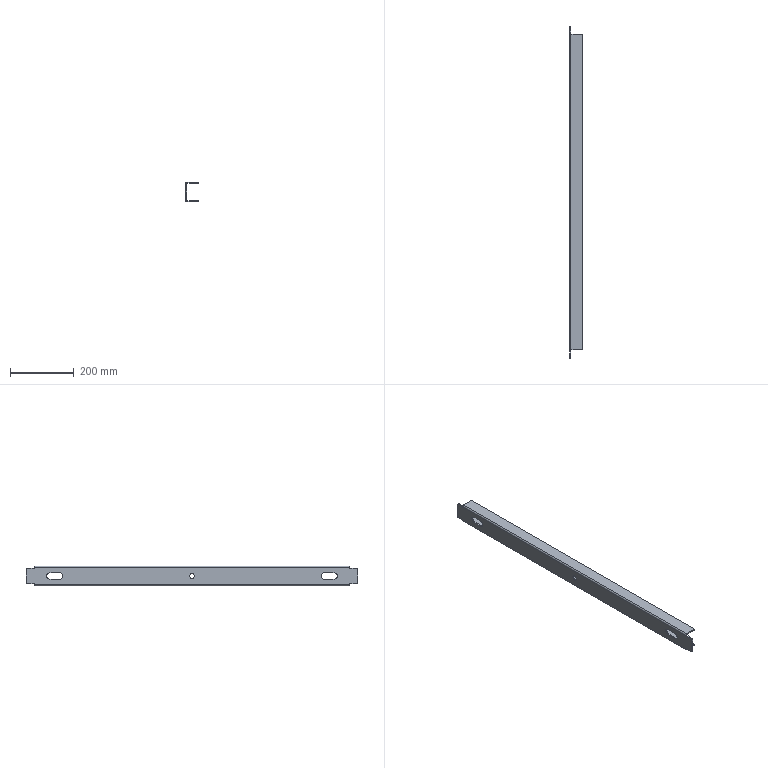Part | SolidWorks | features SMBaseFlange 2, Cut 1, Fillet 1, FlatPattern 1, SheetMetal 1 | 1 solid | 44 faces | box 40 x 1040 x 62 mm | volume 524399 mm3 | plane 30 | cylinder 14 | commonest cylinder face diameters 10 x4 20 x4 0.4 x2 8.4 x2 15 x2
STEP:
#1=CARTESIAN_POINT('',(0.,0.,-7.5));
#2=VERTEX_POINT('',#1);
#3=CARTESIAN_POINT('',(0.,0.,7.5));
#4=VERTEX_POINT('',#3);
#5=CARTESIAN_POINT('',(0.,0.,0.));
#6=DIRECTION('',(-1.,0.,0.));
#7=DIRECTION('',(0.,0.,1.));
#8=AXIS2_PLACEMENT_3D('',#5,#6,#7);
#9=CIRCLE('',#8,7.5);
#10=EDGE_CURVE('',#2,#4,#9,.T.);
#11=ORIENTED_EDGE('',*,*,#10,.T.);
#12=CARTESIAN_POINT('',(4.,0.,7.5));
#13=VERTEX_POINT('',#12);
#14=CARTESIAN_POINT('',(-6.,0.,7.5));
#15=DIRECTION('',(1.,0.,0.));
#16=VECTOR('',#15,1000.);
#17=LINE('',#14,#16);
#18=EDGE_CURVE('',#4,#13,#17,.T.);
#19=ORIENTED_EDGE('',*,*,#18,.T.);
#20=CARTESIAN_POINT('',(4.,0.,-7.5));
#21=VERTEX_POINT('',#20);
#22=CARTESIAN_POINT('',(4.,0.,0.));
#23=DIRECTION('',(1.,0.,0.));
#24=DIRECTION('',(0.,0.,-1.));
#25=AXIS2_PLACEMENT_3D('',#22,#23,#24);
#26=CIRCLE('',#25,7.5);
#27=EDGE_CURVE('',#13,#21,#26,.T.);
#28=ORIENTED_EDGE('',*,*,#27,.T.);
#29=CARTESIAN_POINT('',(-6.,0.,-7.5));
#30=DIRECTION('',(1.,0.,0.));
#31=VECTOR('',#30,1000.);
#32=LINE('',#29,#31);
#33=EDGE_CURVE('',#2,#21,#32,.T.);
#34=ORIENTED_EDGE('',*,*,#33,.F.);
#35=EDGE_LOOP('',(#11,#19,#28,#34));
#36=FACE_OUTER_BOUND('',#35,.T.);
#37=CARTESIAN_POINT('',(-6.,0.,0.));
#38=DIRECTION('',(1.,0.,0.));
#39=DIRECTION('',(0.,0.,-1.));
#40=AXIS2_PLACEMENT_3D('',#37,#38,#39);
#41=CYLINDRICAL_SURFACE('',#40,7.5);
#42=ADVANCED_FACE('',(#36),#41,.F.);
#43=CARTESIAN_POINT('',(4.,-494.,25.));
#44=VERTEX_POINT('',#43);
#45=CARTESIAN_POINT('',(0.,-494.,25.));
#46=VERTEX_POINT('',#45);
#47=CARTESIAN_POINT('',(4.2,-494.,25.));
#48=DIRECTION('',(-1.,0.,0.));
#49=VECTOR('',#48,1000.);
#50=LINE('',#47,#49);
#51=EDGE_CURVE('',#44,#46,#50,.T.);
#52=ORIENTED_EDGE('',*,*,#51,.F.);
#53=CARTESIAN_POINT('',(4.,-494.,26.8));
#54=VERTEX_POINT('',#53);
#55=CARTESIAN_POINT('',(4.,-494.,-31.));
#56=DIRECTION('',(0.,0.,-1.));
#57=VECTOR('',#56,1000.);
#58=LINE('',#55,#57);
#59=EDGE_CURVE('',#54,#44,#58,.T.);
#60=ORIENTED_EDGE('',*,*,#59,.F.);
#61=CARTESIAN_POINT('',(0.,-494.,26.8));
#62=VERTEX_POINT('',#61);
#63=CARTESIAN_POINT('',(4.,-494.,26.8));
#64=DIRECTION('',(-1.,0.,0.));
#65=VECTOR('',#64,1000.);
#66=LINE('',#63,#65);
#67=EDGE_CURVE('',#54,#62,#66,.T.);
#68=ORIENTED_EDGE('',*,*,#67,.T.);
#69=CARTESIAN_POINT('',(0.,-494.,-31.));
#70=DIRECTION('',(0.,0.,-1.));
#71=VECTOR('',#70,1000.);
#72=LINE('',#69,#71);
#73=EDGE_CURVE('',#62,#46,#72,.T.);
#74=ORIENTED_EDGE('',*,*,#73,.T.);
#75=EDGE_LOOP('',(#52,#60,#68,#74));
#76=FACE_OUTER_BOUND('',#75,.T.);
#77=CARTESIAN_POINT('',(4.2,-494.,-27.));
#78=DIRECTION('',(0.,-1.,0.));
#79=DIRECTION('',(0.,0.,-1.));
#80=AXIS2_PLACEMENT_3D('',#77,#78,#79);
#81=PLANE('',#80);
#82=ADVANCED_FACE('',(#76),#81,.T.);
#83=CARTESIAN_POINT('',(4.,494.,-25.));
#84=VERTEX_POINT('',#83);
#85=CARTESIAN_POINT('',(0.,494.,-25.));
#86=VERTEX_POINT('',#85);
#87=CARTESIAN_POINT('',(4.2,494.,-25.));
#88=DIRECTION('',(-1.,0.,0.));
#89=VECTOR('',#88,1000.);
#90=LINE('',#87,#89);
#91=EDGE_CURVE('',#84,#86,#90,.T.);
#92=ORIENTED_EDGE('',*,*,#91,.F.);
#93=CARTESIAN_POINT('',(4.,494.,-26.8));
#94=VERTEX_POINT('',#93);
#95=CARTESIAN_POINT('',(4.,494.,-31.));
#96=DIRECTION('',(0.,0.,-1.));
#97=VECTOR('',#96,1000.);
#98=LINE('',#95,#97);
#99=EDGE_CURVE('',#84,#94,#98,.T.);
#100=ORIENTED_EDGE('',*,*,#99,.T.);
#101=CARTESIAN_POINT('',(0.,494.,-26.8));
#102=VERTEX_POINT('',#101);
#103=CARTESIAN_POINT('',(4.,494.,-26.8));
#104=DIRECTION('',(-1.,0.,0.));
#105=VECTOR('',#104,1000.);
#106=LINE('',#103,#105);
#107=EDGE_CURVE('',#94,#102,#106,.T.);
#108=ORIENTED_EDGE('',*,*,#107,.T.);
#109=CARTESIAN_POINT('',(0.,494.,-31.));
#110=DIRECTION('',(0.,0.,-1.));
#111=VECTOR('',#110,1000.);
#112=LINE('',#109,#111);
#113=EDGE_CURVE('',#86,#102,#112,.T.);
#114=ORIENTED_EDGE('',*,*,#113,.F.);
#115=EDGE_LOOP('',(#92,#100,#108,#114));
#116=FACE_OUTER_BOUND('',#115,.T.);
#117=CARTESIAN_POINT('',(4.2,494.,27.));
#118=DIRECTION('',(0.,1.,0.));
#119=DIRECTION('',(0.,0.,1.));
#120=AXIS2_PLACEMENT_3D('',#117,#118,#119);
#121=PLANE('',#120);
#122=ADVANCED_FACE('',(#116),#121,.T.);
#123=CARTESIAN_POINT('',(0.,494.,26.8));
#124=VERTEX_POINT('',#123);
#125=CARTESIAN_POINT('',(4.,494.,26.8));
#126=VERTEX_POINT('',#125);
#127=CARTESIAN_POINT('',(0.,494.,26.8));
#128=DIRECTION('',(1.,0.,0.));
#129=VECTOR('',#128,1000.);
#130=LINE('',#127,#129);
#131=EDGE_CURVE('',#124,#126,#130,.T.);
#132=ORIENTED_EDGE('',*,*,#131,.F.);
#133=CARTESIAN_POINT('',(4.2,494.,31.));
#134=VERTEX_POINT('',#133);
#135=CARTESIAN_POINT('',(4.2,494.,26.8));
#136=DIRECTION('',(0.,-1.,0.));
#137=DIRECTION('',(0.,0.,1.));
#138=AXIS2_PLACEMENT_3D('',#135,#136,#137);
#139=CIRCLE('',#138,4.2);
#140=EDGE_CURVE('',#134,#124,#139,.T.);
#141=ORIENTED_EDGE('',*,*,#140,.F.);
#142=CARTESIAN_POINT('',(4.2,494.,27.));
#143=VERTEX_POINT('',#142);
#144=CARTESIAN_POINT('',(4.2,494.,27.));
#145=DIRECTION('',(0.,0.,1.));
#146=VECTOR('',#145,1000.);
#147=LINE('',#144,#146);
#148=EDGE_CURVE('',#143,#134,#147,.T.);
#149=ORIENTED_EDGE('',*,*,#148,.F.);
#150=CARTESIAN_POINT('',(4.2,494.,26.8));
#151=DIRECTION('',(0.,-1.,0.));
#152=DIRECTION('',(1.,0.,0.));
#153=AXIS2_PLACEMENT_3D('',#150,#151,#152);
#154=CIRCLE('',#153,0.2);
#155=EDGE_CURVE('',#143,#126,#154,.T.);
#156=ORIENTED_EDGE('',*,*,#155,.T.);
#157=EDGE_LOOP('',(#132,#141,#149,#156));
#158=FACE_OUTER_BOUND('',#157,.T.);
#159=CARTESIAN_POINT('',(0.,494.,26.8));
#160=DIRECTION('',(0.,1.,0.));
#161=DIRECTION('',(0.,0.,1.));
#162=AXIS2_PLACEMENT_3D('',#159,#160,#161);
#163=PLANE('',#162);
#164=ADVANCED_FACE('',(#158),#163,.T.);
#165=CARTESIAN_POINT('',(0.,494.,25.));
#166=VERTEX_POINT('',#165);
#167=CARTESIAN_POINT('',(4.,494.,25.));
#168=VERTEX_POINT('',#167);
#169=CARTESIAN_POINT('',(4.2,494.,25.));
#170=DIRECTION('',(1.,0.,0.));
#171=VECTOR('',#170,1000.);
#172=LINE('',#169,#171);
#173=EDGE_CURVE('',#166,#168,#172,.T.);
#174=ORIENTED_EDGE('',*,*,#173,.F.);
#175=CARTESIAN_POINT('',(0.,494.,-31.));
#176=DIRECTION('',(0.,0.,-1.));
#177=VECTOR('',#176,1000.);
#178=LINE('',#175,#177);
#179=EDGE_CURVE('',#124,#166,#178,.T.);
#180=ORIENTED_EDGE('',*,*,#179,.F.);
#181=ORIENTED_EDGE('',*,*,#131,.T.);
#182=CARTESIAN_POINT('',(4.,494.,-31.));
#183=DIRECTION('',(0.,0.,-1.));
#184=VECTOR('',#183,1000.);
#185=LINE('',#182,#184);
#186=EDGE_CURVE('',#126,#168,#185,.T.);
#187=ORIENTED_EDGE('',*,*,#186,.T.);
#188=EDGE_LOOP('',(#174,#180,#181,#187));
#189=FACE_OUTER_BOUND('',#188,.T.);
#190=CARTESIAN_POINT('',(4.2,494.,27.));
#191=DIRECTION('',(0.,1.,0.));
#192=DIRECTION('',(0.,0.,1.));
#193=AXIS2_PLACEMENT_3D('',#190,#191,#192);
#194=PLANE('',#193);
#195=ADVANCED_FACE('',(#189),#194,.T.);
#196=CARTESIAN_POINT('',(4.2,-494.,31.));
#197=VERTEX_POINT('',#196);
#198=CARTESIAN_POINT('',(4.2,-494.,27.));
#199=VERTEX_POINT('',#198);
#200=CARTESIAN_POINT('',(4.2,-494.,31.));
#201=DIRECTION('',(0.,0.,-1.));
#202=VECTOR('',#201,1000.);
#203=LINE('',#200,#202);
#204=EDGE_CURVE('',#197,#199,#203,.T.);
#205=ORIENTED_EDGE('',*,*,#204,.F.);
#206=CARTESIAN_POINT('',(4.2,-494.,26.8));
#207=DIRECTION('',(0.,-1.,0.));
#208=DIRECTION('',(0.,0.,1.));
#209=AXIS2_PLACEMENT_3D('',#206,#207,#208);
#210=CIRCLE('',#209,4.2);
#211=EDGE_CURVE('',#197,#62,#210,.T.);
#212=ORIENTED_EDGE('',*,*,#211,.T.);
#213=ORIENTED_EDGE('',*,*,#67,.F.);
#214=CARTESIAN_POINT('',(4.2,-494.,26.8));
#215=DIRECTION('',(0.,-1.,0.));
#216=DIRECTION('',(1.,0.,0.));
#217=AXIS2_PLACEMENT_3D('',#214,#215,#216);
#218=CIRCLE('',#217,0.2);
#219=EDGE_CURVE('',#199,#54,#218,.T.);
#220=ORIENTED_EDGE('',*,*,#219,.F.);
#221=EDGE_LOOP('',(#205,#212,#213,#220));
#222=FACE_OUTER_BOUND('',#221,.T.);
#223=CARTESIAN_POINT('',(4.2,-494.,31.));
#224=DIRECTION('',(0.,-1.,0.));
#225=DIRECTION('',(0.,0.,-1.));
#226=AXIS2_PLACEMENT_3D('',#223,#224,#225);
#227=PLANE('',#226);
#228=ADVANCED_FACE('',(#222),#227,.T.);
#229=CARTESIAN_POINT('',(40.,-494.,31.));
#230=VERTEX_POINT('',#229);
#231=CARTESIAN_POINT('',(0.,-494.,31.));
#232=DIRECTION('',(-1.,0.,0.));
#233=VECTOR('',#232,1000.);
#234=LINE('',#231,#233);
#235=EDGE_CURVE('',#230,#197,#234,.T.);
#236=ORIENTED_EDGE('',*,*,#235,.T.);
#237=ORIENTED_EDGE('',*,*,#204,.T.);
#238=CARTESIAN_POINT('',(40.,-494.,27.));
#239=VERTEX_POINT('',#238);
#240=CARTESIAN_POINT('',(0.,-494.,27.));
#241=DIRECTION('',(-1.,0.,0.));
#242=VECTOR('',#241,1000.);
#243=LINE('',#240,#242);
#244=EDGE_CURVE('',#239,#199,#243,.T.);
#245=ORIENTED_EDGE('',*,*,#244,.F.);
#246=CARTESIAN_POINT('',(40.,-494.,27.));
#247=DIRECTION('',(0.,0.,1.));
#248=VECTOR('',#247,1000.);
#249=LINE('',#246,#248);
#250=EDGE_CURVE('',#239,#230,#249,.T.);
#251=ORIENTED_EDGE('',*,*,#250,.T.);
#252=EDGE_LOOP('',(#236,#237,#245,#251));
#253=FACE_OUTER_BOUND('',#252,.T.);
#254=CARTESIAN_POINT('',(4.,-494.,26.8));
#255=DIRECTION('',(0.,-1.,0.));
#256=DIRECTION('',(0.,0.,-1.));
#257=AXIS2_PLACEMENT_3D('',#254,#255,#256);
#258=PLANE('',#257);
#259=ADVANCED_FACE('',(#253),#258,.T.);
#260=CARTESIAN_POINT('',(4.2,494.,-31.));
#261=VERTEX_POINT('',#260);
#262=CARTESIAN_POINT('',(4.2,494.,-27.));
#263=VERTEX_POINT('',#262);
#264=CARTESIAN_POINT('',(4.2,494.,-31.));
#265=DIRECTION('',(0.,0.,1.));
#266=VECTOR('',#265,1000.);
#267=LINE('',#264,#266);
#268=EDGE_CURVE('',#261,#263,#267,.T.);
#269=ORIENTED_EDGE('',*,*,#268,.F.);
#270=CARTESIAN_POINT('',(4.2,494.,-26.8));
#271=DIRECTION('',(0.,-1.,0.));
#272=DIRECTION('',(0.,0.,1.));
#273=AXIS2_PLACEMENT_3D('',#270,#271,#272);
#274=CIRCLE('',#273,4.2);
#275=EDGE_CURVE('',#102,#261,#274,.T.);
#276=ORIENTED_EDGE('',*,*,#275,.F.);
#277=ORIENTED_EDGE('',*,*,#107,.F.);
#278=CARTESIAN_POINT('',(4.2,494.,-26.8));
#279=DIRECTION('',(0.,-1.,0.));
#280=DIRECTION('',(1.,0.,0.));
#281=AXIS2_PLACEMENT_3D('',#278,#279,#280);
#282=CIRCLE('',#281,0.2);
#283=EDGE_CURVE('',#94,#263,#282,.T.);
#284=ORIENTED_EDGE('',*,*,#283,.T.);
#285=EDGE_LOOP('',(#269,#276,#277,#284));
#286=FACE_OUTER_BOUND('',#285,.T.);
#287=CARTESIAN_POINT('',(4.2,494.,-31.));
#288=DIRECTION('',(0.,1.,0.));
#289=DIRECTION('',(0.,0.,1.));
#290=AXIS2_PLACEMENT_3D('',#287,#288,#289);
#291=PLANE('',#290);
#292=ADVANCED_FACE('',(#286),#291,.T.);
#293=CARTESIAN_POINT('',(40.,494.,-31.));
#294=VERTEX_POINT('',#293);
#295=CARTESIAN_POINT('',(0.,494.,-31.));
#296=DIRECTION('',(1.,0.,0.));
#297=VECTOR('',#296,1000.);
#298=LINE('',#295,#297);
#299=EDGE_CURVE('',#261,#294,#298,.T.);
#300=ORIENTED_EDGE('',*,*,#299,.F.);
#301=ORIENTED_EDGE('',*,*,#268,.T.);
#302=CARTESIAN_POINT('',(40.,494.,-27.));
#303=VERTEX_POINT('',#302);
#304=CARTESIAN_POINT('',(0.,494.,-27.));
#305=DIRECTION('',(1.,0.,0.));
#306=VECTOR('',#305,1000.);
#307=LINE('',#304,#306);
#308=EDGE_CURVE('',#263,#303,#307,.T.);
#309=ORIENTED_EDGE('',*,*,#308,.T.);
#310=CARTESIAN_POINT('',(40.,494.,-31.));
#311=DIRECTION('',(0.,0.,1.));
#312=VECTOR('',#311,1000.);
#313=LINE('',#310,#312);
#314=EDGE_CURVE('',#294,#303,#313,.T.);
#315=ORIENTED_EDGE('',*,*,#314,.F.);
#316=EDGE_LOOP('',(#300,#301,#309,#315));
#317=FACE_OUTER_BOUND('',#316,.T.);
#318=CARTESIAN_POINT('',(4.,494.,-26.8));
#319=DIRECTION('',(0.,1.,0.));
#320=DIRECTION('',(0.,0.,1.));
#321=AXIS2_PLACEMENT_3D('',#318,#319,#320);
#322=PLANE('',#321);
#323=ADVANCED_FACE('',(#317),#322,.T.);
#324=CARTESIAN_POINT('',(0.,-494.,-26.8));
#325=VERTEX_POINT('',#324);
#326=CARTESIAN_POINT('',(4.,-494.,-26.8));
#327=VERTEX_POINT('',#326);
#328=CARTESIAN_POINT('',(0.,-494.,-26.8));
#329=DIRECTION('',(1.,0.,0.));
#330=VECTOR('',#329,1000.);
#331=LINE('',#328,#330);
#332=EDGE_CURVE('',#325,#327,#331,.T.);
#333=ORIENTED_EDGE('',*,*,#332,.F.);
#334=CARTESIAN_POINT('',(4.2,-494.,-31.));
#335=VERTEX_POINT('',#334);
#336=CARTESIAN_POINT('',(4.2,-494.,-26.8));
#337=DIRECTION('',(0.,-1.,0.));
#338=DIRECTION('',(0.,0.,1.));
#339=AXIS2_PLACEMENT_3D('',#336,#337,#338);
#340=CIRCLE('',#339,4.2);
#341=EDGE_CURVE('',#325,#335,#340,.T.);
#342=ORIENTED_EDGE('',*,*,#341,.T.);
#343=CARTESIAN_POINT('',(4.2,-494.,-27.));
#344=VERTEX_POINT('',#343);
#345=CARTESIAN_POINT('',(4.2,-494.,-27.));
#346=DIRECTION('',(0.,0.,-1.));
#347=VECTOR('',#346,1000.);
#348=LINE('',#345,#347);
#349=EDGE_CURVE('',#344,#335,#348,.T.);
#350=ORIENTED_EDGE('',*,*,#349,.F.);
#351=CARTESIAN_POINT('',(4.2,-494.,-26.8));
#352=DIRECTION('',(0.,-1.,0.));
#353=DIRECTION('',(1.,0.,0.));
#354=AXIS2_PLACEMENT_3D('',#351,#352,#353);
#355=CIRCLE('',#354,0.2);
#356=EDGE_CURVE('',#327,#344,#355,.T.);
#357=ORIENTED_EDGE('',*,*,#356,.F.);
#358=EDGE_LOOP('',(#333,#342,#350,#357));
#359=FACE_OUTER_BOUND('',#358,.T.);
#360=CARTESIAN_POINT('',(0.,-494.,-26.8));
#361=DIRECTION('',(0.,-1.,0.));
#362=DIRECTION('',(0.,0.,-1.));
#363=AXIS2_PLACEMENT_3D('',#360,#361,#362);
#364=PLANE('',#363);
#365=ADVANCED_FACE('',(#359),#364,.T.);
#366=CARTESIAN_POINT('',(0.,-494.,-25.));
#367=VERTEX_POINT('',#366);
#368=CARTESIAN_POINT('',(4.,-494.,-25.));
#369=VERTEX_POINT('',#368);
#370=CARTESIAN_POINT('',(4.2,-494.,-25.));
#371=DIRECTION('',(1.,0.,0.));
#372=VECTOR('',#371,1000.);
#373=LINE('',#370,#372);
#374=EDGE_CURVE('',#367,#369,#373,.T.);
#375=ORIENTED_EDGE('',*,*,#374,.F.);
#376=CARTESIAN_POINT('',(0.,-494.,-31.));
#377=DIRECTION('',(0.,0.,-1.));
#378=VECTOR('',#377,1000.);
#379=LINE('',#376,#378);
#380=EDGE_CURVE('',#367,#325,#379,.T.);
#381=ORIENTED_EDGE('',*,*,#380,.T.);
#382=ORIENTED_EDGE('',*,*,#332,.T.);
#383=CARTESIAN_POINT('',(4.,-494.,-31.));
#384=DIRECTION('',(0.,0.,-1.));
#385=VECTOR('',#384,1000.);
#386=LINE('',#383,#385);
#387=EDGE_CURVE('',#369,#327,#386,.T.);
#388=ORIENTED_EDGE('',*,*,#387,.F.);
#389=EDGE_LOOP('',(#375,#381,#382,#388));
#390=FACE_OUTER_BOUND('',#389,.T.);
#391=CARTESIAN_POINT('',(4.2,-494.,-27.));
#392=DIRECTION('',(0.,-1.,0.));
#393=DIRECTION('',(0.,0.,-1.));
#394=AXIS2_PLACEMENT_3D('',#391,#392,#393);
#395=PLANE('',#394);
#396=ADVANCED_FACE('',(#390),#395,.T.);
#397=CARTESIAN_POINT('',(40.,-494.,-27.));
#398=VERTEX_POINT('',#397);
#399=CARTESIAN_POINT('',(0.,-494.,-27.));
#400=DIRECTION('',(1.,0.,0.));
#401=VECTOR('',#400,1000.);
#402=LINE('',#399,#401);
#403=EDGE_CURVE('',#344,#398,#402,.T.);
#404=ORIENTED_EDGE('',*,*,#403,.T.);
#405=CARTESIAN_POINT('',(40.,494.,-27.));
#406=DIRECTION('',(0.,-1.,0.));
#407=VECTOR('',#406,1000.);
#408=LINE('',#405,#407);
#409=EDGE_CURVE('',#303,#398,#408,.T.);
#410=ORIENTED_EDGE('',*,*,#409,.F.);
#411=ORIENTED_EDGE('',*,*,#308,.F.);
#412=CARTESIAN_POINT('',(4.2,494.,-27.));
#413=DIRECTION('',(0.,-1.,0.));
#414=VECTOR('',#413,1000.);
#415=LINE('',#412,#414);
#416=EDGE_CURVE('',#263,#344,#415,.T.);
#417=ORIENTED_EDGE('',*,*,#416,.T.);
#418=EDGE_LOOP('',(#404,#410,#411,#417));
#419=FACE_OUTER_BOUND('',#418,.T.);
#420=CARTESIAN_POINT('',(0.,494.,-27.));
#421=DIRECTION('',(0.,0.,-1.));
#422=DIRECTION('',(-1.,0.,0.));
#423=AXIS2_PLACEMENT_3D('',#420,#421,#422);
#424=PLANE('',#423);
#425=ADVANCED_FACE('',(#419),#424,.F.);
#426=CARTESIAN_POINT('',(40.,-494.,-31.));
#427=VERTEX_POINT('',#426);
#428=CARTESIAN_POINT('',(40.,-494.,-31.));
#429=DIRECTION('',(0.,0.,1.));
#430=VECTOR('',#429,1000.);
#431=LINE('',#428,#430);
#432=EDGE_CURVE('',#427,#398,#431,.T.);
#433=ORIENTED_EDGE('',*,*,#432,.F.);
#434=CARTESIAN_POINT('',(40.,494.,-31.));
#435=DIRECTION('',(0.,-1.,0.));
#436=VECTOR('',#435,1000.);
#437=LINE('',#434,#436);
#438=EDGE_CURVE('',#294,#427,#437,.T.);
#439=ORIENTED_EDGE('',*,*,#438,.F.);
#440=ORIENTED_EDGE('',*,*,#314,.T.);
#441=ORIENTED_EDGE('',*,*,#409,.T.);
#442=EDGE_LOOP('',(#433,#439,#440,#441));
#443=FACE_OUTER_BOUND('',#442,.T.);
#444=CARTESIAN_POINT('',(40.,494.,-31.));
#445=DIRECTION('',(1.,0.,0.));
#446=DIRECTION('',(0.,0.,-1.));
#447=AXIS2_PLACEMENT_3D('',#444,#445,#446);
#448=PLANE('',#447);
#449=ADVANCED_FACE('',(#443),#448,.T.);
#450=CARTESIAN_POINT('',(0.,-494.,-31.));
#451=DIRECTION('',(1.,0.,0.));
#452=VECTOR('',#451,1000.);
#453=LINE('',#450,#452);
#454=EDGE_CURVE('',#335,#427,#453,.T.);
#455=ORIENTED_EDGE('',*,*,#454,.F.);
#456=CARTESIAN_POINT('',(4.2,494.,-31.));
#457=DIRECTION('',(0.,-1.,0.));
#458=VECTOR('',#457,1000.);
#459=LINE('',#456,#458);
#460=EDGE_CURVE('',#261,#335,#459,.T.);
#461=ORIENTED_EDGE('',*,*,#460,.F.);
#462=ORIENTED_EDGE('',*,*,#299,.T.);
#463=ORIENTED_EDGE('',*,*,#438,.T.);
#464=EDGE_LOOP('',(#455,#461,#462,#463));
#465=FACE_OUTER_BOUND('',#464,.T.);
#466=CARTESIAN_POINT('',(0.,494.,-31.));
#467=DIRECTION('',(0.,0.,-1.));
#468=DIRECTION('',(-1.,0.,0.));
#469=AXIS2_PLACEMENT_3D('',#466,#467,#468);
#470=PLANE('',#469);
#471=ADVANCED_FACE('',(#465),#470,.T.);
#472=ORIENTED_EDGE('',*,*,#341,.F.);
#473=CARTESIAN_POINT('',(0.,494.,-26.8));
#474=DIRECTION('',(0.,-1.,0.));
#475=VECTOR('',#474,1000.);
#476=LINE('',#473,#475);
#477=EDGE_CURVE('',#102,#325,#476,.T.);
#478=ORIENTED_EDGE('',*,*,#477,.F.);
#479=ORIENTED_EDGE('',*,*,#275,.T.);
#480=ORIENTED_EDGE('',*,*,#460,.T.);
#481=EDGE_LOOP('',(#472,#478,#479,#480));
#482=FACE_OUTER_BOUND('',#481,.T.);
#483=CARTESIAN_POINT('',(4.2,494.,-26.8));
#484=DIRECTION('',(0.,-1.,0.));
#485=DIRECTION('',(0.,0.,-1.));
#486=AXIS2_PLACEMENT_3D('',#483,#484,#485);
#487=CYLINDRICAL_SURFACE('',#486,4.2);
#488=ADVANCED_FACE('',(#482),#487,.T.);
#489=CARTESIAN_POINT('',(0.,415.,-10.));
#490=VERTEX_POINT('',#489);
#491=CARTESIAN_POINT('',(0.,415.,10.));
#492=VERTEX_POINT('',#491);
#493=CARTESIAN_POINT('',(0.,415.,0.));
#494=DIRECTION('',(-1.,0.,0.));
#495=DIRECTION('',(0.,0.,1.));
#496=AXIS2_PLACEMENT_3D('',#493,#494,#495);
#497=CIRCLE('',#496,10.);
#498=EDGE_CURVE('',#490,#492,#497,.T.);
#499=ORIENTED_EDGE('',*,*,#498,.F.);
#500=CARTESIAN_POINT('',(0.,445.,-10.));
#501=VERTEX_POINT('',#500);
#502=CARTESIAN_POINT('',(0.,494.,-10.));
#503=DIRECTION('',(0.,-1.,0.));
#504=VECTOR('',#503,1000.);
#505=LINE('',#502,#504);
#506=EDGE_CURVE('',#501,#490,#505,.T.);
#507=ORIENTED_EDGE('',*,*,#506,.F.);
#508=CARTESIAN_POINT('',(0.,445.,10.));
#509=VERTEX_POINT('',#508);
#510=CARTESIAN_POINT('',(0.,445.,0.));
#511=DIRECTION('',(-1.,0.,0.));
#512=DIRECTION('',(0.,0.,1.));
#513=AXIS2_PLACEMENT_3D('',#510,#511,#512);
#514=CIRCLE('',#513,10.);
#515=EDGE_CURVE('',#509,#501,#514,.T.);
#516=ORIENTED_EDGE('',*,*,#515,.F.);
#517=CARTESIAN_POINT('',(0.,494.,10.));
#518=DIRECTION('',(0.,1.,0.));
#519=VECTOR('',#518,1000.);
#520=LINE('',#517,#519);
#521=EDGE_CURVE('',#492,#509,#520,.T.);
#522=ORIENTED_EDGE('',*,*,#521,.F.);
#523=EDGE_LOOP('',(#499,#507,#516,#522));
#524=FACE_BOUND('',#523,.T.);
#525=ORIENTED_EDGE('',*,*,#10,.F.);
#526=CARTESIAN_POINT('',(0.,0.,0.));
#527=DIRECTION('',(-1.,0.,0.));
#528=DIRECTION('',(0.,0.,1.));
#529=AXIS2_PLACEMENT_3D('',#526,#527,#528);
#530=CIRCLE('',#529,7.5);
#531=EDGE_CURVE('',#4,#2,#530,.T.);
#532=ORIENTED_EDGE('',*,*,#531,.F.);
#533=EDGE_LOOP('',(#525,#532));
#534=FACE_BOUND('',#533,.T.);
#535=CARTESIAN_POINT('',(0.,-415.,10.));
#536=VERTEX_POINT('',#535);
#537=CARTESIAN_POINT('',(0.,-415.,-10.));
#538=VERTEX_POINT('',#537);
#539=CARTESIAN_POINT('',(0.,-415.,0.));
#540=DIRECTION('',(-1.,0.,0.));
#541=DIRECTION('',(0.,0.,1.));
#542=AXIS2_PLACEMENT_3D('',#539,#540,#541);
#543=CIRCLE('',#542,10.);
#544=EDGE_CURVE('',#536,#538,#543,.T.);
#545=ORIENTED_EDGE('',*,*,#544,.F.);
#546=CARTESIAN_POINT('',(0.,-445.,10.));
#547=VERTEX_POINT('',#546);
#548=CARTESIAN_POINT('',(0.,494.,10.));
#549=DIRECTION('',(0.,1.,0.));
#550=VECTOR('',#549,1000.);
#551=LINE('',#548,#550);
#552=EDGE_CURVE('',#547,#536,#551,.T.);
#553=ORIENTED_EDGE('',*,*,#552,.F.);
#554=CARTESIAN_POINT('',(0.,-445.,-10.));
#555=VERTEX_POINT('',#554);
#556=CARTESIAN_POINT('',(0.,-445.,0.));
#557=DIRECTION('',(-1.,0.,0.));
#558=DIRECTION('',(0.,0.,1.));
#559=AXIS2_PLACEMENT_3D('',#556,#557,#558);
#560=CIRCLE('',#559,10.);
#561=EDGE_CURVE('',#555,#547,#560,.T.);
#562=ORIENTED_EDGE('',*,*,#561,.F.);
#563=CARTESIAN_POINT('',(0.,494.,-10.));
#564=DIRECTION('',(0.,-1.,0.));
#565=VECTOR('',#564,1000.);
#566=LINE('',#563,#565);
#567=EDGE_CURVE('',#538,#555,#566,.T.);
#568=ORIENTED_EDGE('',*,*,#567,.F.);
#569=EDGE_LOOP('',(#545,#553,#562,#568));
#570=FACE_BOUND('',#569,.T.);
#571=CARTESIAN_POINT('',(0.,-515.,-25.));
#572=VERTEX_POINT('',#571);
#573=CARTESIAN_POINT('',(0.,-520.,-25.));
#574=DIRECTION('',(0.,1.,0.));
#575=VECTOR('',#574,1000.);
#576=LINE('',#573,#575);
#577=EDGE_CURVE('',#572,#367,#576,.T.);
#578=ORIENTED_EDGE('',*,*,#577,.F.);
#579=CARTESIAN_POINT('',(0.,-520.,-20.));
#580=VERTEX_POINT('',#579);
#581=CARTESIAN_POINT('',(0.,-515.,-20.));
#582=DIRECTION('',(-1.,0.,0.));
#583=DIRECTION('',(0.,0.,1.));
#584=AXIS2_PLACEMENT_3D('',#581,#582,#583);
#585=CIRCLE('',#584,5.);
#586=EDGE_CURVE('',#572,#580,#585,.T.);
#587=ORIENTED_EDGE('',*,*,#586,.T.);
#588=CARTESIAN_POINT('',(0.,-520.,20.));
#589=VERTEX_POINT('',#588);
#590=CARTESIAN_POINT('',(0.,-520.,25.));
#591=DIRECTION('',(0.,0.,-1.));
#592=VECTOR('',#591,1000.);
#593=LINE('',#590,#592);
#594=EDGE_CURVE('',#589,#580,#593,.T.);
#595=ORIENTED_EDGE('',*,*,#594,.F.);
#596=CARTESIAN_POINT('',(0.,-515.,25.));
#597=VERTEX_POINT('',#596);
#598=CARTESIAN_POINT('',(0.,-515.,20.));
#599=DIRECTION('',(-1.,0.,0.));
#600=DIRECTION('',(0.,0.,1.));
#601=AXIS2_PLACEMENT_3D('',#598,#599,#600);
#602=CIRCLE('',#601,5.);
#603=EDGE_CURVE('',#589,#597,#602,.T.);
#604=ORIENTED_EDGE('',*,*,#603,.T.);
#605=CARTESIAN_POINT('',(0.,-520.,25.));
#606=DIRECTION('',(0.,-1.,0.));
#607=VECTOR('',#606,1000.);
#608=LINE('',#605,#607);
#609=EDGE_CURVE('',#46,#597,#608,.T.);
#610=ORIENTED_EDGE('',*,*,#609,.F.);
#611=ORIENTED_EDGE('',*,*,#73,.F.);
#612=CARTESIAN_POINT('',(0.,494.,26.8));
#613=DIRECTION('',(0.,-1.,0.));
#614=VECTOR('',#613,1000.);
#615=LINE('',#612,#614);
#616=EDGE_CURVE('',#124,#62,#615,.T.);
#617=ORIENTED_EDGE('',*,*,#616,.F.);
#618=ORIENTED_EDGE('',*,*,#179,.T.);
#619=CARTESIAN_POINT('',(0.,515.,25.));
#620=VERTEX_POINT('',#619);
#621=CARTESIAN_POINT('',(0.,520.,25.));
#622=DIRECTION('',(0.,-1.,0.));
#623=VECTOR('',#622,1000.);
#624=LINE('',#621,#623);
#625=EDGE_CURVE('',#620,#166,#624,.T.);
#626=ORIENTED_EDGE('',*,*,#625,.F.);
#627=CARTESIAN_POINT('',(0.,520.,20.));
#628=VERTEX_POINT('',#627);
#629=CARTESIAN_POINT('',(0.,515.,20.));
#630=DIRECTION('',(-1.,0.,0.));
#631=DIRECTION('',(0.,0.,1.));
#632=AXIS2_PLACEMENT_3D('',#629,#630,#631);
#633=CIRCLE('',#632,5.);
#634=EDGE_CURVE('',#620,#628,#633,.T.);
#635=ORIENTED_EDGE('',*,*,#634,.T.);
#636=CARTESIAN_POINT('',(0.,520.,-20.));
#637=VERTEX_POINT('',#636);
#638=CARTESIAN_POINT('',(0.,520.,25.));
#639=DIRECTION('',(0.,0.,1.));
#640=VECTOR('',#639,1000.);
#641=LINE('',#638,#640);
#642=EDGE_CURVE('',#637,#628,#641,.T.);
#643=ORIENTED_EDGE('',*,*,#642,.F.);
#644=CARTESIAN_POINT('',(0.,515.,-25.));
#645=VERTEX_POINT('',#644);
#646=CARTESIAN_POINT('',(0.,515.,-20.));
#647=DIRECTION('',(-1.,0.,0.));
#648=DIRECTION('',(0.,0.,1.));
#649=AXIS2_PLACEMENT_3D('',#646,#647,#648);
#650=CIRCLE('',#649,5.);
#651=EDGE_CURVE('',#637,#645,#650,.T.);
#652=ORIENTED_EDGE('',*,*,#651,.T.);
#653=CARTESIAN_POINT('',(0.,520.,-25.));
#654=DIRECTION('',(0.,1.,0.));
#655=VECTOR('',#654,1000.);
#656=LINE('',#653,#655);
#657=EDGE_CURVE('',#86,#645,#656,.T.);
#658=ORIENTED_EDGE('',*,*,#657,.F.);
#659=ORIENTED_EDGE('',*,*,#113,.T.);
#660=ORIENTED_EDGE('',*,*,#477,.T.);
#661=ORIENTED_EDGE('',*,*,#380,.F.);
#662=EDGE_LOOP('',(#578,#587,#595,#604,#610,#611,#617,#618,#626,#635,#643,#652,#658,#659,#660,#661));
#663=FACE_OUTER_BOUND('',#662,.T.);
#664=CARTESIAN_POINT('',(0.,494.,-31.));
#665=DIRECTION('',(-1.,0.,0.));
#666=DIRECTION('',(0.,0.,1.));
#667=AXIS2_PLACEMENT_3D('',#664,#665,#666);
#668=PLANE('',#667);
#669=ADVANCED_FACE('',(#524,#534,#570,#663),#668,.T.);
#670=ORIENTED_EDGE('',*,*,#211,.F.);
#671=CARTESIAN_POINT('',(4.2,494.,31.));
#672=DIRECTION('',(0.,-1.,0.));
#673=VECTOR('',#672,1000.);
#674=LINE('',#671,#673);
#675=EDGE_CURVE('',#134,#197,#674,.T.);
#676=ORIENTED_EDGE('',*,*,#675,.F.);
#677=ORIENTED_EDGE('',*,*,#140,.T.);
#678=ORIENTED_EDGE('',*,*,#616,.T.);
#679=EDGE_LOOP('',(#670,#676,#677,#678));
#680=FACE_OUTER_BOUND('',#679,.T.);
#681=CARTESIAN_POINT('',(4.2,494.,26.8));
#682=DIRECTION('',(0.,-1.,0.));
#683=DIRECTION('',(0.,0.,-1.));
#684=AXIS2_PLACEMENT_3D('',#681,#682,#683);
#685=CYLINDRICAL_SURFACE('',#684,4.2);
#686=ADVANCED_FACE('',(#680),#685,.T.);
#687=ORIENTED_EDGE('',*,*,#235,.F.);
#688=CARTESIAN_POINT('',(40.,494.,31.));
#689=VERTEX_POINT('',#688);
#690=CARTESIAN_POINT('',(40.,494.,31.));
#691=DIRECTION('',(0.,-1.,0.));
#692=VECTOR('',#691,1000.);
#693=LINE('',#690,#692);
#694=EDGE_CURVE('',#689,#230,#693,.T.);
#695=ORIENTED_EDGE('',*,*,#694,.F.);
#696=CARTESIAN_POINT('',(0.,494.,31.));
#697=DIRECTION('',(-1.,0.,0.));
#698=VECTOR('',#697,1000.);
#699=LINE('',#696,#698);
#700=EDGE_CURVE('',#689,#134,#699,.T.);
#701=ORIENTED_EDGE('',*,*,#700,.T.);
#702=ORIENTED_EDGE('',*,*,#675,.T.);
#703=EDGE_LOOP('',(#687,#695,#701,#702));
#704=FACE_OUTER_BOUND('',#703,.T.);
#705=CARTESIAN_POINT('',(0.,494.,31.));
#706=DIRECTION('',(0.,0.,1.));
#707=DIRECTION('',(1.,0.,0.));
#708=AXIS2_PLACEMENT_3D('',#705,#706,#707);
#709=PLANE('',#708);
#710=ADVANCED_FACE('',(#704),#709,.T.);
#711=ORIENTED_EDGE('',*,*,#250,.F.);
#712=CARTESIAN_POINT('',(40.,494.,27.));
#713=VERTEX_POINT('',#712);
#714=CARTESIAN_POINT('',(40.,494.,27.));
#715=DIRECTION('',(0.,-1.,0.));
#716=VECTOR('',#715,1000.);
#717=LINE('',#714,#716);
#718=EDGE_CURVE('',#713,#239,#717,.T.);
#719=ORIENTED_EDGE('',*,*,#718,.F.);
#720=CARTESIAN_POINT('',(40.,494.,27.));
#721=DIRECTION('',(0.,0.,1.));
#722=VECTOR('',#721,1000.);
#723=LINE('',#720,#722);
#724=EDGE_CURVE('',#713,#689,#723,.T.);
#725=ORIENTED_EDGE('',*,*,#724,.T.);
#726=ORIENTED_EDGE('',*,*,#694,.T.);
#727=EDGE_LOOP('',(#711,#719,#725,#726));
#728=FACE_OUTER_BOUND('',#727,.T.);
#729=CARTESIAN_POINT('',(40.,494.,27.));
#730=DIRECTION('',(1.,0.,0.));
#731=DIRECTION('',(0.,0.,-1.));
#732=AXIS2_PLACEMENT_3D('',#729,#730,#731);
#733=PLANE('',#732);
#734=ADVANCED_FACE('',(#728),#733,.T.);
#735=ORIENTED_EDGE('',*,*,#244,.T.);
#736=CARTESIAN_POINT('',(4.2,494.,27.));
#737=DIRECTION('',(0.,-1.,0.));
#738=VECTOR('',#737,1000.);
#739=LINE('',#736,#738);
#740=EDGE_CURVE('',#143,#199,#739,.T.);
#741=ORIENTED_EDGE('',*,*,#740,.F.);
#742=CARTESIAN_POINT('',(0.,494.,27.));
#743=DIRECTION('',(-1.,0.,0.));
#744=VECTOR('',#743,1000.);
#745=LINE('',#742,#744);
#746=EDGE_CURVE('',#713,#143,#745,.T.);
#747=ORIENTED_EDGE('',*,*,#746,.F.);
#748=ORIENTED_EDGE('',*,*,#718,.T.);
#749=EDGE_LOOP('',(#735,#741,#747,#748));
#750=FACE_OUTER_BOUND('',#749,.T.);
#751=CARTESIAN_POINT('',(0.,494.,27.));
#752=DIRECTION('',(0.,0.,1.));
#753=DIRECTION('',(1.,0.,0.));
#754=AXIS2_PLACEMENT_3D('',#751,#752,#753);
#755=PLANE('',#754);
#756=ADVANCED_FACE('',(#750),#755,.F.);
#757=ORIENTED_EDGE('',*,*,#219,.T.);
#758=CARTESIAN_POINT('',(4.,494.,26.8));
#759=DIRECTION('',(0.,-1.,0.));
#760=VECTOR('',#759,1000.);
#761=LINE('',#758,#760);
#762=EDGE_CURVE('',#126,#54,#761,.T.);
#763=ORIENTED_EDGE('',*,*,#762,.F.);
#764=ORIENTED_EDGE('',*,*,#155,.F.);
#765=ORIENTED_EDGE('',*,*,#740,.T.);
#766=EDGE_LOOP('',(#757,#763,#764,#765));
#767=FACE_OUTER_BOUND('',#766,.T.);
#768=CARTESIAN_POINT('',(4.2,494.,26.8));
#769=DIRECTION('',(0.,-1.,0.));
#770=DIRECTION('',(0.,0.,-1.));
#771=AXIS2_PLACEMENT_3D('',#768,#769,#770);
#772=CYLINDRICAL_SURFACE('',#771,0.2);
#773=ADVANCED_FACE('',(#767),#772,.F.);
#774=CARTESIAN_POINT('',(4.,415.,-10.));
#775=VERTEX_POINT('',#774);
#776=CARTESIAN_POINT('',(4.,445.,-10.));
#777=VERTEX_POINT('',#776);
#778=CARTESIAN_POINT('',(4.,415.,-10.));
#779=DIRECTION('',(0.,1.,0.));
#780=VECTOR('',#779,1000.);
#781=LINE('',#778,#780);
#782=EDGE_CURVE('',#775,#777,#781,.T.);
#783=ORIENTED_EDGE('',*,*,#782,.F.);
#784=CARTESIAN_POINT('',(4.,415.,10.));
#785=VERTEX_POINT('',#784);
#786=CARTESIAN_POINT('',(4.,415.,0.));
#787=DIRECTION('',(1.,0.,0.));
#788=DIRECTION('',(0.,0.,-1.));
#789=AXIS2_PLACEMENT_3D('',#786,#787,#788);
#790=CIRCLE('',#789,10.);
#791=EDGE_CURVE('',#785,#775,#790,.T.);
#792=ORIENTED_EDGE('',*,*,#791,.F.);
#793=CARTESIAN_POINT('',(4.,445.,10.));
#794=VERTEX_POINT('',#793);
#795=CARTESIAN_POINT('',(4.,415.,10.));
#796=DIRECTION('',(0.,-1.,0.));
#797=VECTOR('',#796,1000.);
#798=LINE('',#795,#797);
#799=EDGE_CURVE('',#794,#785,#798,.T.);
#800=ORIENTED_EDGE('',*,*,#799,.F.);
#801=CARTESIAN_POINT('',(4.,445.,0.));
#802=DIRECTION('',(1.,0.,0.));
#803=DIRECTION('',(0.,0.,-1.));
#804=AXIS2_PLACEMENT_3D('',#801,#802,#803);
#805=CIRCLE('',#804,10.);
#806=EDGE_CURVE('',#777,#794,#805,.T.);
#807=ORIENTED_EDGE('',*,*,#806,.F.);
#808=EDGE_LOOP('',(#783,#792,#800,#807));
#809=FACE_BOUND('',#808,.T.);
#810=CARTESIAN_POINT('',(4.,0.,0.));
#811=DIRECTION('',(1.,0.,0.));
#812=DIRECTION('',(0.,0.,-1.));
#813=AXIS2_PLACEMENT_3D('',#810,#811,#812);
#814=CIRCLE('',#813,7.5);
#815=EDGE_CURVE('',#21,#13,#814,.T.);
#816=ORIENTED_EDGE('',*,*,#815,.F.);
#817=ORIENTED_EDGE('',*,*,#27,.F.);
#818=EDGE_LOOP('',(#816,#817));
#819=FACE_BOUND('',#818,.T.);
#820=CARTESIAN_POINT('',(4.,-415.,10.));
#821=VERTEX_POINT('',#820);
#822=CARTESIAN_POINT('',(4.,-445.,10.));
#823=VERTEX_POINT('',#822);
#824=CARTESIAN_POINT('',(4.,-415.,10.));
#825=DIRECTION('',(0.,-1.,0.));
#826=VECTOR('',#825,1000.);
#827=LINE('',#824,#826);
#828=EDGE_CURVE('',#821,#823,#827,.T.);
#829=ORIENTED_EDGE('',*,*,#828,.F.);
#830=CARTESIAN_POINT('',(4.,-415.,-10.));
#831=VERTEX_POINT('',#830);
#832=CARTESIAN_POINT('',(4.,-415.,0.));
#833=DIRECTION('',(1.,0.,0.));
#834=DIRECTION('',(0.,0.,1.));
#835=AXIS2_PLACEMENT_3D('',#832,#833,#834);
#836=CIRCLE('',#835,10.);
#837=EDGE_CURVE('',#831,#821,#836,.T.);
#838=ORIENTED_EDGE('',*,*,#837,.F.);
#839=CARTESIAN_POINT('',(4.,-445.,-10.));
#840=VERTEX_POINT('',#839);
#841=CARTESIAN_POINT('',(4.,-415.,-10.));
#842=DIRECTION('',(0.,1.,0.));
#843=VECTOR('',#842,1000.);
#844=LINE('',#841,#843);
#845=EDGE_CURVE('',#840,#831,#844,.T.);
#846=ORIENTED_EDGE('',*,*,#845,.F.);
#847=CARTESIAN_POINT('',(4.,-445.,0.));
#848=DIRECTION('',(1.,0.,0.));
#849=DIRECTION('',(0.,0.,1.));
#850=AXIS2_PLACEMENT_3D('',#847,#848,#849);
#851=CIRCLE('',#850,10.);
#852=EDGE_CURVE('',#823,#840,#851,.T.);
#853=ORIENTED_EDGE('',*,*,#852,.F.);
#854=EDGE_LOOP('',(#829,#838,#846,#853));
#855=FACE_BOUND('',#854,.T.);
#856=CARTESIAN_POINT('',(4.,-520.,20.));
#857=VERTEX_POINT('',#856);
#858=CARTESIAN_POINT('',(4.,-520.,-20.));
#859=VERTEX_POINT('',#858);
#860=CARTESIAN_POINT('',(4.,-520.,25.));
#861=DIRECTION('',(0.,0.,-1.));
#862=VECTOR('',#861,1000.);
#863=LINE('',#860,#862);
#864=EDGE_CURVE('',#857,#859,#863,.T.);
#865=ORIENTED_EDGE('',*,*,#864,.T.);
#866=CARTESIAN_POINT('',(4.,-515.,-25.));
#867=VERTEX_POINT('',#866);
#868=CARTESIAN_POINT('',(4.,-515.,-20.));
#869=DIRECTION('',(1.,0.,0.));
#870=DIRECTION('',(0.,0.,1.));
#871=AXIS2_PLACEMENT_3D('',#868,#869,#870);
#872=CIRCLE('',#871,5.);
#873=EDGE_CURVE('',#859,#867,#872,.T.);
#874=ORIENTED_EDGE('',*,*,#873,.T.);
#875=CARTESIAN_POINT('',(4.,-520.,-25.));
#876=DIRECTION('',(0.,1.,0.));
#877=VECTOR('',#876,1000.);
#878=LINE('',#875,#877);
#879=EDGE_CURVE('',#867,#369,#878,.T.);
#880=ORIENTED_EDGE('',*,*,#879,.T.);
#881=ORIENTED_EDGE('',*,*,#387,.T.);
#882=CARTESIAN_POINT('',(4.,494.,-26.8));
#883=DIRECTION('',(0.,-1.,0.));
#884=VECTOR('',#883,1000.);
#885=LINE('',#882,#884);
#886=EDGE_CURVE('',#94,#327,#885,.T.);
#887=ORIENTED_EDGE('',*,*,#886,.F.);
#888=ORIENTED_EDGE('',*,*,#99,.F.);
#889=CARTESIAN_POINT('',(4.,515.,-25.));
#890=VERTEX_POINT('',#889);
#891=CARTESIAN_POINT('',(4.,520.,-25.));
#892=DIRECTION('',(0.,1.,0.));
#893=VECTOR('',#892,1000.);
#894=LINE('',#891,#893);
#895=EDGE_CURVE('',#84,#890,#894,.T.);
#896=ORIENTED_EDGE('',*,*,#895,.T.);
#897=CARTESIAN_POINT('',(4.,520.,-20.));
#898=VERTEX_POINT('',#897);
#899=CARTESIAN_POINT('',(4.,515.,-20.));
#900=DIRECTION('',(1.,0.,0.));
#901=DIRECTION('',(0.,0.,1.));
#902=AXIS2_PLACEMENT_3D('',#899,#900,#901);
#903=CIRCLE('',#902,5.);
#904=EDGE_CURVE('',#890,#898,#903,.T.);
#905=ORIENTED_EDGE('',*,*,#904,.T.);
#906=CARTESIAN_POINT('',(4.,520.,20.));
#907=VERTEX_POINT('',#906);
#908=CARTESIAN_POINT('',(4.,520.,25.));
#909=DIRECTION('',(0.,0.,1.));
#910=VECTOR('',#909,1000.);
#911=LINE('',#908,#910);
#912=EDGE_CURVE('',#898,#907,#911,.T.);
#913=ORIENTED_EDGE('',*,*,#912,.T.);
#914=CARTESIAN_POINT('',(4.,515.,25.));
#915=VERTEX_POINT('',#914);
#916=CARTESIAN_POINT('',(4.,515.,20.));
#917=DIRECTION('',(1.,0.,0.));
#918=DIRECTION('',(0.,0.,1.));
#919=AXIS2_PLACEMENT_3D('',#916,#917,#918);
#920=CIRCLE('',#919,5.);
#921=EDGE_CURVE('',#907,#915,#920,.T.);
#922=ORIENTED_EDGE('',*,*,#921,.T.);
#923=CARTESIAN_POINT('',(4.,520.,25.));
#924=DIRECTION('',(0.,-1.,0.));
#925=VECTOR('',#924,1000.);
#926=LINE('',#923,#925);
#927=EDGE_CURVE('',#915,#168,#926,.T.);
#928=ORIENTED_EDGE('',*,*,#927,.T.);
#929=ORIENTED_EDGE('',*,*,#186,.F.);
#930=ORIENTED_EDGE('',*,*,#762,.T.);
#931=ORIENTED_EDGE('',*,*,#59,.T.);
#932=CARTESIAN_POINT('',(4.,-515.,25.));
#933=VERTEX_POINT('',#932);
#934=CARTESIAN_POINT('',(4.,-520.,25.));
#935=DIRECTION('',(0.,-1.,0.));
#936=VECTOR('',#935,1000.);
#937=LINE('',#934,#936);
#938=EDGE_CURVE('',#44,#933,#937,.T.);
#939=ORIENTED_EDGE('',*,*,#938,.T.);
#940=CARTESIAN_POINT('',(4.,-515.,20.));
#941=DIRECTION('',(1.,0.,0.));
#942=DIRECTION('',(0.,0.,1.));
#943=AXIS2_PLACEMENT_3D('',#940,#941,#942);
#944=CIRCLE('',#943,5.);
#945=EDGE_CURVE('',#933,#857,#944,.T.);
#946=ORIENTED_EDGE('',*,*,#945,.T.);
#947=EDGE_LOOP('',(#865,#874,#880,#881,#887,#888,#896,#905,#913,#922,#928,#929,#930,#931,#939,#946));
#948=FACE_OUTER_BOUND('',#947,.T.);
#949=CARTESIAN_POINT('',(4.,494.,-31.));
#950=DIRECTION('',(-1.,0.,0.));
#951=DIRECTION('',(0.,0.,1.));
#952=AXIS2_PLACEMENT_3D('',#949,#950,#951);
#953=PLANE('',#952);
#954=ADVANCED_FACE('',(#809,#819,#855,#948),#953,.F.);
#955=ORIENTED_EDGE('',*,*,#356,.T.);
#956=ORIENTED_EDGE('',*,*,#416,.F.);
#957=ORIENTED_EDGE('',*,*,#283,.F.);
#958=ORIENTED_EDGE('',*,*,#886,.T.);
#959=EDGE_LOOP('',(#955,#956,#957,#958));
#960=FACE_OUTER_BOUND('',#959,.T.);
#961=CARTESIAN_POINT('',(4.2,494.,-26.8));
#962=DIRECTION('',(0.,-1.,0.));
#963=DIRECTION('',(0.,0.,-1.));
#964=AXIS2_PLACEMENT_3D('',#961,#962,#963);
#965=CYLINDRICAL_SURFACE('',#964,0.2);
#966=ADVANCED_FACE('',(#960),#965,.F.);
#967=ORIENTED_EDGE('',*,*,#746,.T.);
#968=ORIENTED_EDGE('',*,*,#148,.T.);
#969=ORIENTED_EDGE('',*,*,#700,.F.);
#970=ORIENTED_EDGE('',*,*,#724,.F.);
#971=EDGE_LOOP('',(#967,#968,#969,#970));
#972=FACE_OUTER_BOUND('',#971,.T.);
#973=CARTESIAN_POINT('',(4.2,494.,-26.8));
#974=DIRECTION('',(0.,1.,0.));
#975=DIRECTION('',(1.,0.,0.));
#976=AXIS2_PLACEMENT_3D('',#973,#974,#975);
#977=PLANE('',#976);
#978=ADVANCED_FACE('',(#972),#977,.T.);
#979=ORIENTED_EDGE('',*,*,#403,.F.);
#980=ORIENTED_EDGE('',*,*,#349,.T.);
#981=ORIENTED_EDGE('',*,*,#454,.T.);
#982=ORIENTED_EDGE('',*,*,#432,.T.);
#983=EDGE_LOOP('',(#979,#980,#981,#982));
#984=FACE_OUTER_BOUND('',#983,.T.);
#985=CARTESIAN_POINT('',(4.2,-494.,-26.8));
#986=DIRECTION('',(0.,1.,0.));
#987=DIRECTION('',(1.,0.,0.));
#988=AXIS2_PLACEMENT_3D('',#985,#986,#987);
#989=PLANE('',#988);
#990=ADVANCED_FACE('',(#984),#989,.F.);
#991=ORIENTED_EDGE('',*,*,#657,.T.);
#992=CARTESIAN_POINT('',(0.,515.,-25.));
#993=DIRECTION('',(1.,0.,0.));
#994=VECTOR('',#993,1000.);
#995=LINE('',#992,#994);
#996=EDGE_CURVE('',#645,#890,#995,.T.);
#997=ORIENTED_EDGE('',*,*,#996,.T.);
#998=ORIENTED_EDGE('',*,*,#895,.F.);
#999=ORIENTED_EDGE('',*,*,#91,.T.);
#1000=EDGE_LOOP('',(#991,#997,#998,#999));
#1001=FACE_OUTER_BOUND('',#1000,.T.);
#1002=CARTESIAN_POINT('',(0.,520.,-25.));
#1003=DIRECTION('',(0.,0.,-1.));
#1004=DIRECTION('',(-1.,0.,0.));
#1005=AXIS2_PLACEMENT_3D('',#1002,#1003,#1004);
#1006=PLANE('',#1005);
#1007=ADVANCED_FACE('',(#1001),#1006,.T.);
#1008=ORIENTED_EDGE('',*,*,#927,.F.);
#1009=CARTESIAN_POINT('',(0.,515.,25.));
#1010=DIRECTION('',(-1.,0.,0.));
#1011=VECTOR('',#1010,1000.);
#1012=LINE('',#1009,#1011);
#1013=EDGE_CURVE('',#915,#620,#1012,.T.);
#1014=ORIENTED_EDGE('',*,*,#1013,.T.);
#1015=ORIENTED_EDGE('',*,*,#625,.T.);
#1016=ORIENTED_EDGE('',*,*,#173,.T.);
#1017=EDGE_LOOP('',(#1008,#1014,#1015,#1016));
#1018=FACE_OUTER_BOUND('',#1017,.T.);
#1019=CARTESIAN_POINT('',(0.,520.,25.));
#1020=DIRECTION('',(0.,0.,1.));
#1021=DIRECTION('',(1.,0.,0.));
#1022=AXIS2_PLACEMENT_3D('',#1019,#1020,#1021);
#1023=PLANE('',#1022);
#1024=ADVANCED_FACE('',(#1018),#1023,.T.);
#1025=ORIENTED_EDGE('',*,*,#642,.T.);
#1026=CARTESIAN_POINT('',(0.,520.,20.));
#1027=DIRECTION('',(1.,0.,0.));
#1028=VECTOR('',#1027,1000.);
#1029=LINE('',#1026,#1028);
#1030=EDGE_CURVE('',#628,#907,#1029,.T.);
#1031=ORIENTED_EDGE('',*,*,#1030,.T.);
#1032=ORIENTED_EDGE('',*,*,#912,.F.);
#1033=CARTESIAN_POINT('',(0.,520.,-20.));
#1034=DIRECTION('',(-1.,0.,0.));
#1035=VECTOR('',#1034,1000.);
#1036=LINE('',#1033,#1035);
#1037=EDGE_CURVE('',#898,#637,#1036,.T.);
#1038=ORIENTED_EDGE('',*,*,#1037,.T.);
#1039=EDGE_LOOP('',(#1025,#1031,#1032,#1038));
#1040=FACE_OUTER_BOUND('',#1039,.T.);
#1041=CARTESIAN_POINT('',(0.,520.,25.));
#1042=DIRECTION('',(0.,1.,0.));
#1043=DIRECTION('',(0.,0.,1.));
#1044=AXIS2_PLACEMENT_3D('',#1041,#1042,#1043);
#1045=PLANE('',#1044);
#1046=ADVANCED_FACE('',(#1040),#1045,.T.);
#1047=ORIENTED_EDGE('',*,*,#609,.T.);
#1048=CARTESIAN_POINT('',(0.,-515.,25.));
#1049=DIRECTION('',(1.,0.,0.));
#1050=VECTOR('',#1049,1000.);
#1051=LINE('',#1048,#1050);
#1052=EDGE_CURVE('',#597,#933,#1051,.T.);
#1053=ORIENTED_EDGE('',*,*,#1052,.T.);
#1054=ORIENTED_EDGE('',*,*,#938,.F.);
#1055=ORIENTED_EDGE('',*,*,#51,.T.);
#1056=EDGE_LOOP('',(#1047,#1053,#1054,#1055));
#1057=FACE_OUTER_BOUND('',#1056,.T.);
#1058=CARTESIAN_POINT('',(0.,-520.,25.));
#1059=DIRECTION('',(0.,0.,1.));
#1060=DIRECTION('',(1.,0.,0.));
#1061=AXIS2_PLACEMENT_3D('',#1058,#1059,#1060);
#1062=PLANE('',#1061);
#1063=ADVANCED_FACE('',(#1057),#1062,.T.);
#1064=ORIENTED_EDGE('',*,*,#879,.F.);
#1065=CARTESIAN_POINT('',(0.,-515.,-25.));
#1066=DIRECTION('',(-1.,0.,0.));
#1067=VECTOR('',#1066,1000.);
#1068=LINE('',#1065,#1067);
#1069=EDGE_CURVE('',#867,#572,#1068,.T.);
#1070=ORIENTED_EDGE('',*,*,#1069,.T.);
#1071=ORIENTED_EDGE('',*,*,#577,.T.);
#1072=ORIENTED_EDGE('',*,*,#374,.T.);
#1073=EDGE_LOOP('',(#1064,#1070,#1071,#1072));
#1074=FACE_OUTER_BOUND('',#1073,.T.);
#1075=CARTESIAN_POINT('',(0.,-520.,-25.));
#1076=DIRECTION('',(0.,0.,-1.));
#1077=DIRECTION('',(-1.,0.,0.));
#1078=AXIS2_PLACEMENT_3D('',#1075,#1076,#1077);
#1079=PLANE('',#1078);
#1080=ADVANCED_FACE('',(#1074),#1079,.T.);
#1081=ORIENTED_EDGE('',*,*,#594,.T.);
#1082=CARTESIAN_POINT('',(0.,-520.,-20.));
#1083=DIRECTION('',(1.,0.,0.));
#1084=VECTOR('',#1083,1000.);
#1085=LINE('',#1082,#1084);
#1086=EDGE_CURVE('',#580,#859,#1085,.T.);
#1087=ORIENTED_EDGE('',*,*,#1086,.T.);
#1088=ORIENTED_EDGE('',*,*,#864,.F.);
#1089=CARTESIAN_POINT('',(0.,-520.,20.));
#1090=DIRECTION('',(-1.,0.,0.));
#1091=VECTOR('',#1090,1000.);
#1092=LINE('',#1089,#1091);
#1093=EDGE_CURVE('',#857,#589,#1092,.T.);
#1094=ORIENTED_EDGE('',*,*,#1093,.T.);
#1095=EDGE_LOOP('',(#1081,#1087,#1088,#1094));
#1096=FACE_OUTER_BOUND('',#1095,.T.);
#1097=CARTESIAN_POINT('',(0.,-520.,25.));
#1098=DIRECTION('',(0.,-1.,0.));
#1099=DIRECTION('',(0.,0.,-1.));
#1100=AXIS2_PLACEMENT_3D('',#1097,#1098,#1099);
#1101=PLANE('',#1100);
#1102=ADVANCED_FACE('',(#1096),#1101,.T.);
#1103=ORIENTED_EDGE('',*,*,#586,.F.);
#1104=ORIENTED_EDGE('',*,*,#1069,.F.);
#1105=ORIENTED_EDGE('',*,*,#873,.F.);
#1106=ORIENTED_EDGE('',*,*,#1086,.F.);
#1107=EDGE_LOOP('',(#1103,#1104,#1105,#1106));
#1108=FACE_OUTER_BOUND('',#1107,.T.);
#1109=CARTESIAN_POINT('',(0.,-515.,-20.));
#1110=DIRECTION('',(1.,0.,0.));
#1111=DIRECTION('',(0.,0.,-1.));
#1112=AXIS2_PLACEMENT_3D('',#1109,#1110,#1111);
#1113=CYLINDRICAL_SURFACE('',#1112,5.);
#1114=ADVANCED_FACE('',(#1108),#1113,.T.);
#1115=ORIENTED_EDGE('',*,*,#603,.F.);
#1116=ORIENTED_EDGE('',*,*,#1093,.F.);
#1117=ORIENTED_EDGE('',*,*,#945,.F.);
#1118=ORIENTED_EDGE('',*,*,#1052,.F.);
#1119=EDGE_LOOP('',(#1115,#1116,#1117,#1118));
#1120=FACE_OUTER_BOUND('',#1119,.T.);
#1121=CARTESIAN_POINT('',(0.,-515.,20.));
#1122=DIRECTION('',(1.,0.,0.));
#1123=DIRECTION('',(0.,0.,-1.));
#1124=AXIS2_PLACEMENT_3D('',#1121,#1122,#1123);
#1125=CYLINDRICAL_SURFACE('',#1124,5.);
#1126=ADVANCED_FACE('',(#1120),#1125,.T.);
#1127=ORIENTED_EDGE('',*,*,#634,.F.);
#1128=ORIENTED_EDGE('',*,*,#1013,.F.);
#1129=ORIENTED_EDGE('',*,*,#921,.F.);
#1130=ORIENTED_EDGE('',*,*,#1030,.F.);
#1131=EDGE_LOOP('',(#1127,#1128,#1129,#1130));
#1132=FACE_OUTER_BOUND('',#1131,.T.);
#1133=CARTESIAN_POINT('',(0.,515.,20.));
#1134=DIRECTION('',(1.,0.,0.));
#1135=DIRECTION('',(0.,0.,-1.));
#1136=AXIS2_PLACEMENT_3D('',#1133,#1134,#1135);
#1137=CYLINDRICAL_SURFACE('',#1136,5.);
#1138=ADVANCED_FACE('',(#1132),#1137,.T.);
#1139=ORIENTED_EDGE('',*,*,#651,.F.);
#1140=ORIENTED_EDGE('',*,*,#1037,.F.);
#1141=ORIENTED_EDGE('',*,*,#904,.F.);
#1142=ORIENTED_EDGE('',*,*,#996,.F.);
#1143=EDGE_LOOP('',(#1139,#1140,#1141,#1142));
#1144=FACE_OUTER_BOUND('',#1143,.T.);
#1145=CARTESIAN_POINT('',(0.,515.,-20.));
#1146=DIRECTION('',(1.,0.,0.));
#1147=DIRECTION('',(0.,0.,-1.));
#1148=AXIS2_PLACEMENT_3D('',#1145,#1146,#1147);
#1149=CYLINDRICAL_SURFACE('',#1148,5.);
#1150=ADVANCED_FACE('',(#1144),#1149,.T.);
#1151=ORIENTED_EDGE('',*,*,#544,.T.);
#1152=CARTESIAN_POINT('',(-6.,-415.,-10.));
#1153=DIRECTION('',(1.,0.,0.));
#1154=VECTOR('',#1153,1000.);
#1155=LINE('',#1152,#1154);
#1156=EDGE_CURVE('',#538,#831,#1155,.T.);
#1157=ORIENTED_EDGE('',*,*,#1156,.T.);
#1158=ORIENTED_EDGE('',*,*,#837,.T.);
#1159=CARTESIAN_POINT('',(-6.,-415.,10.));
#1160=DIRECTION('',(1.,0.,0.));
#1161=VECTOR('',#1160,1000.);
#1162=LINE('',#1159,#1161);
#1163=EDGE_CURVE('',#536,#821,#1162,.T.);
#1164=ORIENTED_EDGE('',*,*,#1163,.F.);
#1165=EDGE_LOOP('',(#1151,#1157,#1158,#1164));
#1166=FACE_OUTER_BOUND('',#1165,.T.);
#1167=CARTESIAN_POINT('',(-6.,-415.,0.));
#1168=DIRECTION('',(1.,0.,0.));
#1169=DIRECTION('',(0.,0.,-1.));
#1170=AXIS2_PLACEMENT_3D('',#1167,#1168,#1169);
#1171=CYLINDRICAL_SURFACE('',#1170,10.);
#1172=ADVANCED_FACE('',(#1166),#1171,.F.);
#1173=ORIENTED_EDGE('',*,*,#567,.T.);
#1174=CARTESIAN_POINT('',(-6.,-445.,-10.));
#1175=DIRECTION('',(1.,0.,0.));
#1176=VECTOR('',#1175,1000.);
#1177=LINE('',#1174,#1176);
#1178=EDGE_CURVE('',#555,#840,#1177,.T.);
#1179=ORIENTED_EDGE('',*,*,#1178,.T.);
#1180=ORIENTED_EDGE('',*,*,#845,.T.);
#1181=ORIENTED_EDGE('',*,*,#1156,.F.);
#1182=EDGE_LOOP('',(#1173,#1179,#1180,#1181));
#1183=FACE_OUTER_BOUND('',#1182,.T.);
#1184=CARTESIAN_POINT('',(-6.,-415.,-10.));
#1185=DIRECTION('',(0.,0.,-1.));
#1186=DIRECTION('',(-1.,0.,0.));
#1187=AXIS2_PLACEMENT_3D('',#1184,#1185,#1186);
#1188=PLANE('',#1187);
#1189=ADVANCED_FACE('',(#1183),#1188,.F.);
#1190=ORIENTED_EDGE('',*,*,#561,.T.);
#1191=CARTESIAN_POINT('',(-6.,-445.,10.));
#1192=DIRECTION('',(1.,0.,0.));
#1193=VECTOR('',#1192,1000.);
#1194=LINE('',#1191,#1193);
#1195=EDGE_CURVE('',#547,#823,#1194,.T.);
#1196=ORIENTED_EDGE('',*,*,#1195,.T.);
#1197=ORIENTED_EDGE('',*,*,#852,.T.);
#1198=ORIENTED_EDGE('',*,*,#1178,.F.);
#1199=EDGE_LOOP('',(#1190,#1196,#1197,#1198));
#1200=FACE_OUTER_BOUND('',#1199,.T.);
#1201=CARTESIAN_POINT('',(-6.,-445.,0.));
#1202=DIRECTION('',(1.,0.,0.));
#1203=DIRECTION('',(0.,0.,-1.));
#1204=AXIS2_PLACEMENT_3D('',#1201,#1202,#1203);
#1205=CYLINDRICAL_SURFACE('',#1204,10.);
#1206=ADVANCED_FACE('',(#1200),#1205,.F.);
#1207=ORIENTED_EDGE('',*,*,#552,.T.);
#1208=ORIENTED_EDGE('',*,*,#1163,.T.);
#1209=ORIENTED_EDGE('',*,*,#828,.T.);
#1210=ORIENTED_EDGE('',*,*,#1195,.F.);
#1211=EDGE_LOOP('',(#1207,#1208,#1209,#1210));
#1212=FACE_OUTER_BOUND('',#1211,.T.);
#1213=CARTESIAN_POINT('',(-6.,-415.,10.));
#1214=DIRECTION('',(0.,0.,1.));
#1215=DIRECTION('',(1.,0.,0.));
#1216=AXIS2_PLACEMENT_3D('',#1213,#1214,#1215);
#1217=PLANE('',#1216);
#1218=ADVANCED_FACE('',(#1212),#1217,.F.);
#1219=ORIENTED_EDGE('',*,*,#18,.F.);
#1220=ORIENTED_EDGE('',*,*,#531,.T.);
#1221=ORIENTED_EDGE('',*,*,#33,.T.);
#1222=ORIENTED_EDGE('',*,*,#815,.T.);
#1223=EDGE_LOOP('',(#1219,#1220,#1221,#1222));
#1224=FACE_OUTER_BOUND('',#1223,.T.);
#1225=CARTESIAN_POINT('',(-6.,0.,0.));
#1226=DIRECTION('',(1.,0.,0.));
#1227=DIRECTION('',(0.,0.,-1.));
#1228=AXIS2_PLACEMENT_3D('',#1225,#1226,#1227);
#1229=CYLINDRICAL_SURFACE('',#1228,7.5);
#1230=ADVANCED_FACE('',(#1224),#1229,.F.);
#1231=ORIENTED_EDGE('',*,*,#498,.T.);
#1232=CARTESIAN_POINT('',(-6.,415.,10.));
#1233=DIRECTION('',(1.,0.,0.));
#1234=VECTOR('',#1233,1000.);
#1235=LINE('',#1232,#1234);
#1236=EDGE_CURVE('',#492,#785,#1235,.T.);
#1237=ORIENTED_EDGE('',*,*,#1236,.T.);
#1238=ORIENTED_EDGE('',*,*,#791,.T.);
#1239=CARTESIAN_POINT('',(-6.,415.,-10.));
#1240=DIRECTION('',(1.,0.,0.));
#1241=VECTOR('',#1240,1000.);
#1242=LINE('',#1239,#1241);
#1243=EDGE_CURVE('',#490,#775,#1242,.T.);
#1244=ORIENTED_EDGE('',*,*,#1243,.F.);
#1245=EDGE_LOOP('',(#1231,#1237,#1238,#1244));
#1246=FACE_OUTER_BOUND('',#1245,.T.);
#1247=CARTESIAN_POINT('',(-6.,415.,0.));
#1248=DIRECTION('',(1.,0.,0.));
#1249=DIRECTION('',(0.,0.,-1.));
#1250=AXIS2_PLACEMENT_3D('',#1247,#1248,#1249);
#1251=CYLINDRICAL_SURFACE('',#1250,10.);
#1252=ADVANCED_FACE('',(#1246),#1251,.F.);
#1253=ORIENTED_EDGE('',*,*,#521,.T.);
#1254=CARTESIAN_POINT('',(-6.,445.,10.));
#1255=DIRECTION('',(1.,0.,0.));
#1256=VECTOR('',#1255,1000.);
#1257=LINE('',#1254,#1256);
#1258=EDGE_CURVE('',#509,#794,#1257,.T.);
#1259=ORIENTED_EDGE('',*,*,#1258,.T.);
#1260=ORIENTED_EDGE('',*,*,#799,.T.);
#1261=ORIENTED_EDGE('',*,*,#1236,.F.);
#1262=EDGE_LOOP('',(#1253,#1259,#1260,#1261));
#1263=FACE_OUTER_BOUND('',#1262,.T.);
#1264=CARTESIAN_POINT('',(-6.,415.,10.));
#1265=DIRECTION('',(0.,0.,1.));
#1266=DIRECTION('',(1.,0.,0.));
#1267=AXIS2_PLACEMENT_3D('',#1264,#1265,#1266);
#1268=PLANE('',#1267);
#1269=ADVANCED_FACE('',(#1263),#1268,.F.);
#1270=ORIENTED_EDGE('',*,*,#515,.T.);
#1271=CARTESIAN_POINT('',(-6.,445.,-10.));
#1272=DIRECTION('',(1.,0.,0.));
#1273=VECTOR('',#1272,1000.);
#1274=LINE('',#1271,#1273);
#1275=EDGE_CURVE('',#501,#777,#1274,.T.);
#1276=ORIENTED_EDGE('',*,*,#1275,.T.);
#1277=ORIENTED_EDGE('',*,*,#806,.T.);
#1278=ORIENTED_EDGE('',*,*,#1258,.F.);
#1279=EDGE_LOOP('',(#1270,#1276,#1277,#1278));
#1280=FACE_OUTER_BOUND('',#1279,.T.);
#1281=CARTESIAN_POINT('',(-6.,445.,0.));
#1282=DIRECTION('',(1.,0.,0.));
#1283=DIRECTION('',(0.,0.,-1.));
#1284=AXIS2_PLACEMENT_3D('',#1281,#1282,#1283);
#1285=CYLINDRICAL_SURFACE('',#1284,10.);
#1286=ADVANCED_FACE('',(#1280),#1285,.F.);
#1287=ORIENTED_EDGE('',*,*,#506,.T.);
#1288=ORIENTED_EDGE('',*,*,#1243,.T.);
#1289=ORIENTED_EDGE('',*,*,#782,.T.);
#1290=ORIENTED_EDGE('',*,*,#1275,.F.);
#1291=EDGE_LOOP('',(#1287,#1288,#1289,#1290));
#1292=FACE_OUTER_BOUND('',#1291,.T.);
#1293=CARTESIAN_POINT('',(-6.,415.,-10.));
#1294=DIRECTION('',(0.,0.,-1.));
#1295=DIRECTION('',(-1.,0.,0.));
#1296=AXIS2_PLACEMENT_3D('',#1293,#1294,#1295);
#1297=PLANE('',#1296);
#1298=ADVANCED_FACE('',(#1292),#1297,.F.);
#1299=CLOSED_SHELL('',(#42,#82,#122,#164,#195,#228,#259,#292,#323,#365,#396,#425,#449,#471,#488,#669,#686,#710,#734,#756,#773,#954,#966,#978,#990,#1007,#1024,#1046,#1063,#1080,#1102,#1114,#1126,#1138,#1150,#1172,#1189,#1206,#1218,#1230,#1252,#1269,#1286,#1298));
#1300=MANIFOLD_SOLID_BREP('',#1299);
#1301=CARTESIAN_POINT('',(0.,0.,0.));
#1302=DIRECTION('',(0.,0.,1.));
#1303=DIRECTION('',(1.,0.,0.));
#1304=AXIS2_PLACEMENT_3D('',#1301,#1302,#1303);
#1305=(LENGTH_UNIT()NAMED_UNIT(*)SI_UNIT(.MILLI.,.METRE.));
#1306=UNCERTAINTY_MEASURE_WITH_UNIT(LENGTH_MEASURE(0.00001),#1305,'','');
#1307=(NAMED_UNIT(*)PLANE_ANGLE_UNIT()SI_UNIT($,.RADIAN.));
#1308=(NAMED_UNIT(*)SI_UNIT($,.STERADIAN.)SOLID_ANGLE_UNIT());
#1309=(GEOMETRIC_REPRESENTATION_CONTEXT(3)GLOBAL_UNCERTAINTY_ASSIGNED_CONTEXT((#1306))GLOBAL_UNIT_ASSIGNED_CONTEXT((#1305,#1307,#1308))REPRESENTATION_CONTEXT('',''));
#1310=ADVANCED_BREP_SHAPE_REPRESENTATION('',(#1300,#1304),#1309);